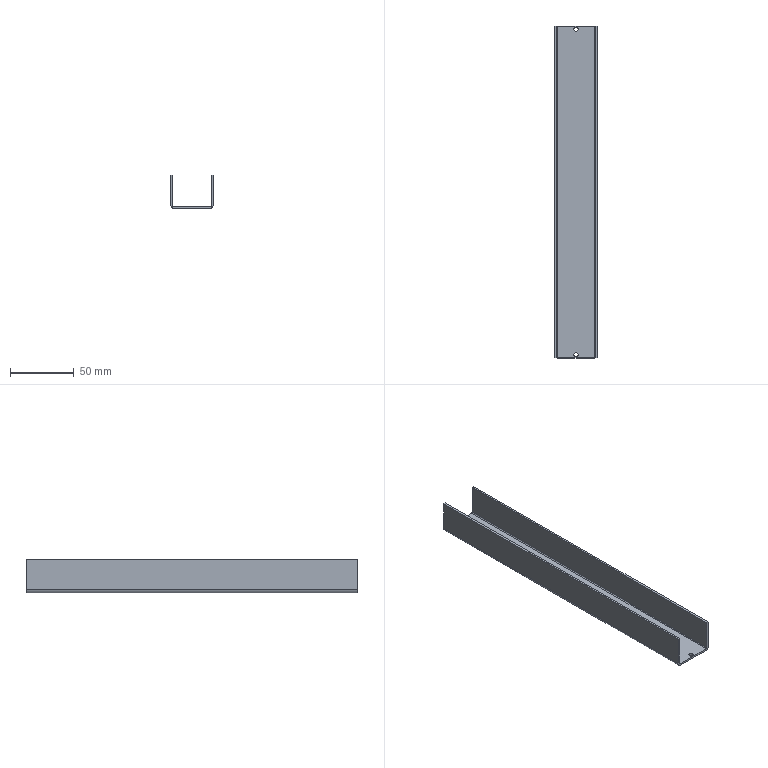Part | STEP file | PN_0067 Mount electronic clip s horizontal manipulator upper cover | 1 solid | 26 faces | box 33 x 260 x 26 mm | volume 31457 mm3 | plane 18 | cylinder 8 | commonest cylinder face diameters 3.3 x4 1.473 x2 4.473 x2